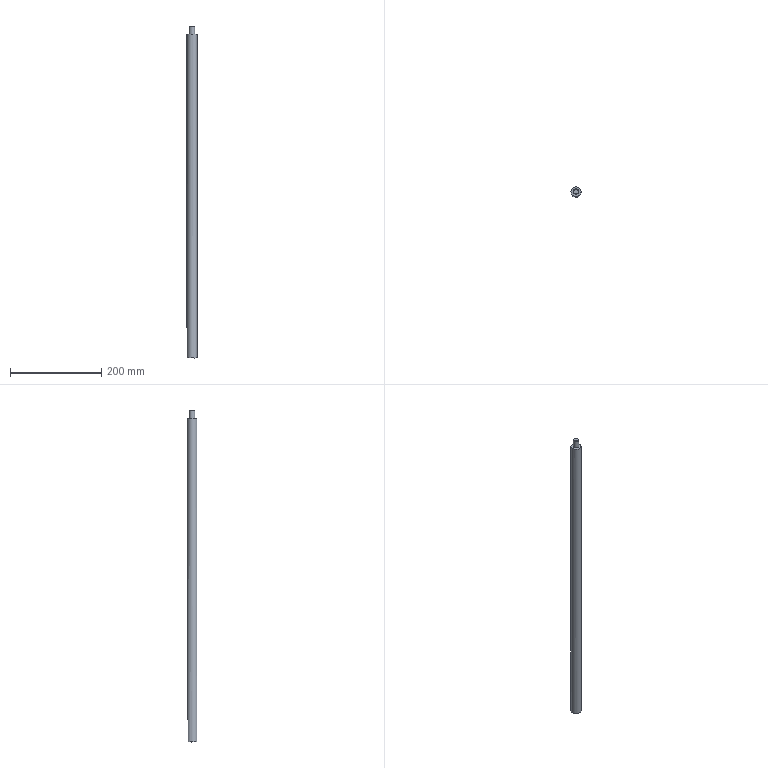Part | STEP file | solid 236 | 1 solid | 11 faces | box 22 x 22 x 728.65 mm | volume 268884 mm3 | plane 5 | cylinder 3 | cone 3 | commonest cylinder face diameters 10.2 x1 12 x1 22 x1